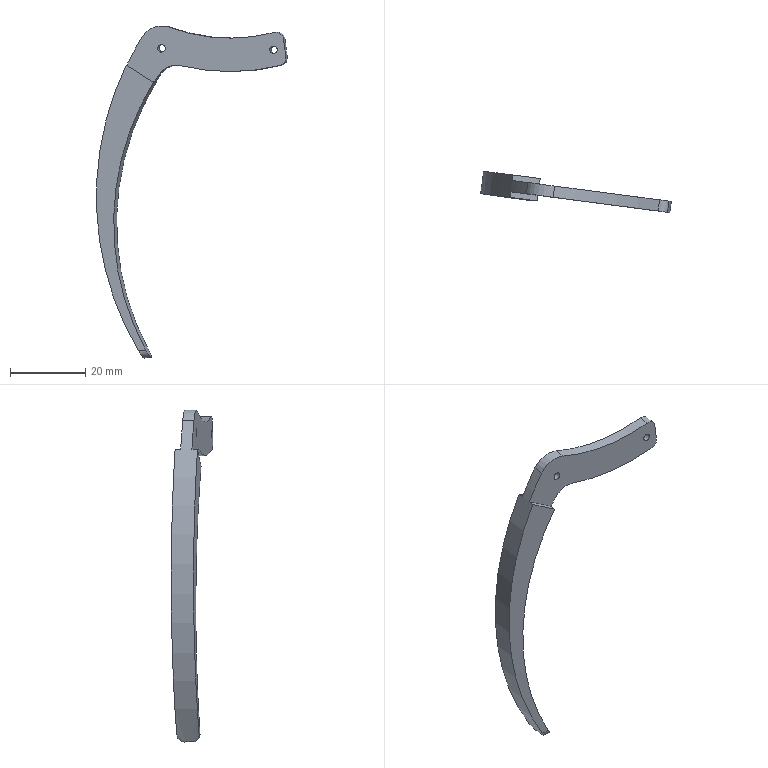Part | NX | features DATUM_CSYS 4, EXTRUDE 3, SKETCH 3, CPROJ 2, BLEND 1 | 1 solid | 20 faces | box 50.786 x 11.051 x 88.315 mm | volume 3379 mm3 | cylinder 12 | plane 8 | commonest cylinder face diameters 4 x4 2 x2 10.7 x1 12 x1 94.72 x1 112.5 x1
STEP:
#1=CARTESIAN_POINT('',(-233.818,36.549,339.632));
#2=VERTEX_POINT('',#1);
#3=CARTESIAN_POINT('',(-237.962,37.093,332.031));
#4=VERTEX_POINT('',#3);
#5=CARTESIAN_POINT('',(-166.053,27.654,297.099));
#6=DIRECTION('',(0.1302,0.9915,-0.000002994));
#7=DIRECTION('',(-0.9915,0.1302,0.));
#8=AXIS2_PLACEMENT_3D('',#5,#6,#7);
#9=CIRCLE('',#8,80.5);
#10=EDGE_CURVE('',#2,#4,#9,.F.);
#11=ORIENTED_EDGE('',*,*,#10,.T.);
#12=CARTESIAN_POINT('',(-237.767,38.58,332.031));
#13=VERTEX_POINT('',#12);
#14=CARTESIAN_POINT('',(-238.547,32.631,332.031));
#15=DIRECTION('',(0.1302,0.9915,-0.000002994));
#16=VECTOR('',#15,1000.);
#17=LINE('',#14,#16);
#18=EDGE_CURVE('',#4,#13,#17,.T.);
#19=ORIENTED_EDGE('',*,*,#18,.T.);
#20=CARTESIAN_POINT('',(-234.495,38.151,256.014));
#21=VERTEX_POINT('',#20);
#22=CARTESIAN_POINT('',(-165.858,29.141,297.099));
#23=DIRECTION('',(0.1302,0.9915,-0.000002994));
#24=DIRECTION('',(0.9915,-0.1302,0.));
#25=AXIS2_PLACEMENT_3D('',#22,#23,#24);
#26=CIRCLE('',#25,80.5);
#27=EDGE_CURVE('',#21,#13,#26,.T.);
#28=ORIENTED_EDGE('',*,*,#27,.F.);
#29=CARTESIAN_POINT('',(-233.623,36.019,254.147));
#30=VERTEX_POINT('',#29);
#31=CARTESIAN_POINT('',(-234.495,38.151,256.014));
#32=CARTESIAN_POINT('',(-234.215,38.114,255.539));
#33=CARTESIAN_POINT('',(-233.699,37.656,254.602));
#34=CARTESIAN_POINT('',(-233.55,36.569,254.147));
#35=CARTESIAN_POINT('',(-233.623,36.019,254.147));
#36=B_SPLINE_CURVE_WITH_KNOTS('',3,(#31,#32,#33,#34,#35),.UNSPECIFIED.,.F.,.F.,(4,1,4),(0.,0.001636,0.003273),.UNSPECIFIED.);
#37=EDGE_CURVE('',#21,#30,#36,.T.);
#38=ORIENTED_EDGE('',*,*,#37,.T.);
#39=CARTESIAN_POINT('',(-233.883,34.036,254.147));
#40=VERTEX_POINT('',#39);
#41=CARTESIAN_POINT('',(-234.143,32.053,254.147));
#42=DIRECTION('',(0.1302,0.9915,-0.000002994));
#43=VECTOR('',#42,1000.);
#44=LINE('',#41,#43);
#45=EDGE_CURVE('',#40,#30,#44,.T.);
#46=ORIENTED_EDGE('',*,*,#45,.F.);
#47=CARTESIAN_POINT('',(-235.276,32.202,256.014));
#48=VERTEX_POINT('',#47);
#49=CARTESIAN_POINT('',(-233.883,34.036,254.147));
#50=CARTESIAN_POINT('',(-233.955,33.487,254.147));
#51=CARTESIAN_POINT('',(-234.378,32.476,254.6));
#52=CARTESIAN_POINT('',(-234.997,32.165,255.539));
#53=CARTESIAN_POINT('',(-235.276,32.202,256.014));
#54=B_SPLINE_CURVE_WITH_KNOTS('',3,(#49,#50,#51,#52,#53),.UNSPECIFIED.,.F.,.F.,(4,1,4),(0.,0.001636,0.003273),.UNSPECIFIED.);
#55=EDGE_CURVE('',#40,#48,#54,.T.);
#56=ORIENTED_EDGE('',*,*,#55,.T.);
#57=CARTESIAN_POINT('',(-238.547,32.631,332.031));
#58=VERTEX_POINT('',#57);
#59=CARTESIAN_POINT('',(-166.639,23.192,297.099));
#60=DIRECTION('',(0.1302,0.9915,-0.000002994));
#61=DIRECTION('',(0.9915,-0.1302,0.));
#62=AXIS2_PLACEMENT_3D('',#59,#60,#61);
#63=CIRCLE('',#62,80.5);
#64=EDGE_CURVE('',#48,#58,#63,.T.);
#65=ORIENTED_EDGE('',*,*,#64,.T.);
#66=CARTESIAN_POINT('',(-238.352,34.119,332.031));
#67=VERTEX_POINT('',#66);
#68=CARTESIAN_POINT('',(-238.547,32.631,332.031));
#69=DIRECTION('',(0.1302,0.9915,-0.000002994));
#70=VECTOR('',#69,1000.);
#71=LINE('',#68,#70);
#72=EDGE_CURVE('',#67,#58,#71,.F.);
#73=ORIENTED_EDGE('',*,*,#72,.F.);
#74=CARTESIAN_POINT('',(-234.208,33.575,339.632));
#75=VERTEX_POINT('',#74);
#76=CARTESIAN_POINT('',(-166.443,24.679,297.099));
#77=DIRECTION('',(0.1302,0.9915,-0.000002994));
#78=DIRECTION('',(-0.9915,0.1302,0.));
#79=AXIS2_PLACEMENT_3D('',#76,#77,#78);
#80=CIRCLE('',#79,80.5);
#81=EDGE_CURVE('',#75,#67,#80,.F.);
#82=ORIENTED_EDGE('',*,*,#81,.F.);
#83=CARTESIAN_POINT('',(-234.403,32.087,339.632));
#84=DIRECTION('',(0.1302,0.9915,-0.000002994));
#85=VECTOR('',#84,1000.);
#86=LINE('',#83,#85);
#87=EDGE_CURVE('',#75,#2,#86,.T.);
#88=ORIENTED_EDGE('',*,*,#87,.T.);
#89=EDGE_LOOP('',(#11,#19,#28,#38,#46,#56,#65,#73,#82,#88));
#90=FACE_BOUND('',#89,.T.);
#91=CARTESIAN_POINT('',(-166.639,23.192,297.099));
#92=DIRECTION('',(0.1302,0.9915,-0.000002994));
#93=DIRECTION('',(-0.9915,0.1302,0.));
#94=AXIS2_PLACEMENT_3D('',#91,#92,#93);
#95=CYLINDRICAL_SURFACE('',#94,80.5);
#96=ADVANCED_FACE('',(#90),#95,.T.);
#97=CARTESIAN_POINT('',(-227.109,32.643,342.095));
#98=VERTEX_POINT('',#97);
#99=CARTESIAN_POINT('',(-226.718,35.617,342.095));
#100=VERTEX_POINT('',#99);
#101=CARTESIAN_POINT('',(-227.304,31.156,342.095));
#102=DIRECTION('',(0.1302,0.9915,-0.000002994));
#103=VECTOR('',#102,1000.);
#104=LINE('',#101,#103);
#105=EDGE_CURVE('',#98,#100,#104,.T.);
#106=ORIENTED_EDGE('',*,*,#105,.T.);
#107=CARTESIAN_POINT('',(-228.767,35.886,336.462));
#108=DIRECTION('',(0.1302,0.9915,-0.000002994));
#109=DIRECTION('',(-0.9915,0.1302,0.));
#110=AXIS2_PLACEMENT_3D('',#107,#108,#109);
#111=CIRCLE('',#110,6.);
#112=EDGE_CURVE('',#100,#2,#111,.F.);
#113=ORIENTED_EDGE('',*,*,#112,.T.);
#114=ORIENTED_EDGE('',*,*,#87,.F.);
#115=CARTESIAN_POINT('',(-229.157,32.912,336.462));
#116=DIRECTION('',(0.1302,0.9915,-0.000002994));
#117=DIRECTION('',(-0.9915,0.1302,0.));
#118=AXIS2_PLACEMENT_3D('',#115,#116,#117);
#119=CIRCLE('',#118,6.);
#120=EDGE_CURVE('',#98,#75,#119,.F.);
#121=ORIENTED_EDGE('',*,*,#120,.F.);
#122=EDGE_LOOP('',(#106,#113,#114,#121));
#123=FACE_BOUND('',#122,.T.);
#124=CARTESIAN_POINT('',(-229.352,31.424,336.462));
#125=DIRECTION('',(0.1302,0.9915,-0.000002994));
#126=DIRECTION('',(-0.9915,0.1302,0.));
#127=AXIS2_PLACEMENT_3D('',#124,#125,#126);
#128=CYLINDRICAL_SURFACE('',#127,6.);
#129=ADVANCED_FACE('',(#123),#128,.T.);
#130=CARTESIAN_POINT('',(-199.174,28.976,340.71));
#131=VERTEX_POINT('',#130);
#132=CARTESIAN_POINT('',(-198.783,31.95,340.71));
#133=VERTEX_POINT('',#132);
#134=CARTESIAN_POINT('',(-199.369,27.488,340.71));
#135=DIRECTION('',(0.1302,0.9915,-0.000002994));
#136=VECTOR('',#135,1000.);
#137=LINE('',#134,#136);
#138=EDGE_CURVE('',#131,#133,#137,.T.);
#139=ORIENTED_EDGE('',*,*,#138,.T.);
#140=CARTESIAN_POINT('',(-210.55,33.495,386.559));
#141=DIRECTION('',(0.1302,0.9915,-0.000002994));
#142=DIRECTION('',(-0.9915,0.1302,0.));
#143=AXIS2_PLACEMENT_3D('',#140,#141,#142);
#144=CIRCLE('',#143,47.36);
#145=EDGE_CURVE('',#133,#100,#144,.T.);
#146=ORIENTED_EDGE('',*,*,#145,.T.);
#147=ORIENTED_EDGE('',*,*,#105,.F.);
#148=CARTESIAN_POINT('',(-210.94,30.521,386.559));
#149=DIRECTION('',(0.1302,0.9915,-0.000002994));
#150=DIRECTION('',(-0.9915,0.1302,0.));
#151=AXIS2_PLACEMENT_3D('',#148,#149,#150);
#152=CIRCLE('',#151,47.36);
#153=EDGE_CURVE('',#131,#98,#152,.T.);
#154=ORIENTED_EDGE('',*,*,#153,.F.);
#155=EDGE_LOOP('',(#139,#146,#147,#154));
#156=FACE_BOUND('',#155,.T.);
#157=CARTESIAN_POINT('',(-211.135,29.033,386.559));
#158=DIRECTION('',(0.1302,0.9915,-0.000002994));
#159=DIRECTION('',(-0.9915,0.1302,0.));
#160=AXIS2_PLACEMENT_3D('',#157,#158,#159);
#161=CYLINDRICAL_SURFACE('',#160,47.36);
#162=ADVANCED_FACE('',(#156),#161,.F.);
#163=CARTESIAN_POINT('',(-196.71,28.652,339.034));
#164=VERTEX_POINT('',#163);
#165=CARTESIAN_POINT('',(-196.32,31.627,339.034));
#166=VERTEX_POINT('',#165);
#167=CARTESIAN_POINT('',(-196.906,27.165,339.034));
#168=DIRECTION('',(0.1302,0.9915,-0.000002994));
#169=VECTOR('',#168,1000.);
#170=LINE('',#167,#169);
#171=EDGE_CURVE('',#164,#166,#170,.T.);
#172=ORIENTED_EDGE('',*,*,#171,.T.);
#173=CARTESIAN_POINT('',(-198.286,31.885,338.774));
#174=DIRECTION('',(0.1302,0.9915,-0.000002994));
#175=DIRECTION('',(-0.9915,0.1302,0.));
#176=AXIS2_PLACEMENT_3D('',#173,#174,#175);
#177=CIRCLE('',#176,2.);
#178=EDGE_CURVE('',#166,#133,#177,.F.);
#179=ORIENTED_EDGE('',*,*,#178,.T.);
#180=ORIENTED_EDGE('',*,*,#138,.F.);
#181=CARTESIAN_POINT('',(-198.677,28.911,338.774));
#182=DIRECTION('',(0.1302,0.9915,-0.000002994));
#183=DIRECTION('',(-0.9915,0.1302,0.));
#184=AXIS2_PLACEMENT_3D('',#181,#182,#183);
#185=CIRCLE('',#184,2.);
#186=EDGE_CURVE('',#164,#131,#185,.F.);
#187=ORIENTED_EDGE('',*,*,#186,.F.);
#188=EDGE_LOOP('',(#172,#179,#180,#187));
#189=FACE_BOUND('',#188,.T.);
#190=CARTESIAN_POINT('',(-198.872,27.423,338.774));
#191=DIRECTION('',(0.1302,0.9915,-0.000002994));
#192=DIRECTION('',(-0.9915,0.1302,0.));
#193=AXIS2_PLACEMENT_3D('',#190,#191,#192);
#194=CYLINDRICAL_SURFACE('',#193,2.);
#195=ADVANCED_FACE('',(#189),#194,.T.);
#196=CARTESIAN_POINT('',(-196.075,28.569,334.153));
#197=VERTEX_POINT('',#196);
#198=CARTESIAN_POINT('',(-195.685,31.543,334.153));
#199=VERTEX_POINT('',#198);
#200=CARTESIAN_POINT('',(-196.27,27.082,334.153));
#201=DIRECTION('',(0.1302,0.9915,-0.000002994));
#202=VECTOR('',#201,1000.);
#203=LINE('',#200,#202);
#204=EDGE_CURVE('',#197,#199,#203,.T.);
#205=ORIENTED_EDGE('',*,*,#204,.T.);
#206=CARTESIAN_POINT('',(-196.32,31.627,339.034));
#207=DIRECTION('',(-0.129,0.01694,0.9915));
#208=VECTOR('',#207,1000.);
#209=LINE('',#206,#208);
#210=EDGE_CURVE('',#199,#166,#209,.T.);
#211=ORIENTED_EDGE('',*,*,#210,.T.);
#212=ORIENTED_EDGE('',*,*,#171,.F.);
#213=CARTESIAN_POINT('',(-196.71,28.652,339.034));
#214=DIRECTION('',(-0.129,0.01694,0.9915));
#215=VECTOR('',#214,1000.);
#216=LINE('',#213,#215);
#217=EDGE_CURVE('',#197,#164,#216,.T.);
#218=ORIENTED_EDGE('',*,*,#217,.F.);
#219=EDGE_LOOP('',(#205,#211,#212,#218));
#220=FACE_BOUND('',#219,.T.);
#221=CARTESIAN_POINT('',(-196.906,27.165,339.034));
#222=DIRECTION('',(0.9831,-0.129,0.1302));
#223=DIRECTION('',(0.1313,0.,-0.9913));
#224=AXIS2_PLACEMENT_3D('',#221,#222,#223);
#225=PLANE('',#224);
#226=ADVANCED_FACE('',(#220),#225,.T.);
#227=CARTESIAN_POINT('',(-197.566,28.765,331.951));
#228=VERTEX_POINT('',#227);
#229=CARTESIAN_POINT('',(-197.175,31.739,331.951));
#230=VERTEX_POINT('',#229);
#231=CARTESIAN_POINT('',(-197.761,27.277,331.951));
#232=DIRECTION('',(0.1302,0.9915,-0.000002994));
#233=VECTOR('',#232,1000.);
#234=LINE('',#231,#233);
#235=EDGE_CURVE('',#228,#230,#234,.T.);
#236=ORIENTED_EDGE('',*,*,#235,.T.);
#237=CARTESIAN_POINT('',(-197.651,31.802,333.892));
#238=DIRECTION('',(0.1302,0.9915,-0.000002994));
#239=DIRECTION('',(-0.9915,0.1302,0.));
#240=AXIS2_PLACEMENT_3D('',#237,#238,#239);
#241=CIRCLE('',#240,2.);
#242=EDGE_CURVE('',#230,#199,#241,.F.);
#243=ORIENTED_EDGE('',*,*,#242,.T.);
#244=ORIENTED_EDGE('',*,*,#204,.F.);
#245=CARTESIAN_POINT('',(-198.041,28.827,333.892));
#246=DIRECTION('',(0.1302,0.9915,-0.000002994));
#247=DIRECTION('',(-0.9915,0.1302,0.));
#248=AXIS2_PLACEMENT_3D('',#245,#246,#247);
#249=CIRCLE('',#248,2.);
#250=EDGE_CURVE('',#228,#197,#249,.F.);
#251=ORIENTED_EDGE('',*,*,#250,.F.);
#252=EDGE_LOOP('',(#236,#243,#244,#251));
#253=FACE_BOUND('',#252,.T.);
#254=CARTESIAN_POINT('',(-198.236,27.34,333.892));
#255=DIRECTION('',(0.1302,0.9915,-0.000002994));
#256=DIRECTION('',(-0.9915,0.1302,0.));
#257=AXIS2_PLACEMENT_3D('',#254,#255,#256);
#258=CYLINDRICAL_SURFACE('',#257,2.);
#259=ADVANCED_FACE('',(#253),#258,.T.);
#260=CARTESIAN_POINT('',(-224.029,32.239,331.88));
#261=VERTEX_POINT('',#260);
#262=CARTESIAN_POINT('',(-223.639,35.213,331.88));
#263=VERTEX_POINT('',#262);
#264=CARTESIAN_POINT('',(-224.225,30.751,331.88));
#265=DIRECTION('',(0.1302,0.9915,-0.000002994));
#266=VECTOR('',#265,1000.);
#267=LINE('',#264,#266);
#268=EDGE_CURVE('',#261,#263,#267,.T.);
#269=ORIENTED_EDGE('',*,*,#268,.T.);
#270=CARTESIAN_POINT('',(-210.55,33.495,386.559));
#271=DIRECTION('',(0.1302,0.9915,-0.000002994));
#272=DIRECTION('',(-0.9915,0.1302,0.));
#273=AXIS2_PLACEMENT_3D('',#270,#271,#272);
#274=CIRCLE('',#273,56.25);
#275=EDGE_CURVE('',#263,#230,#274,.F.);
#276=ORIENTED_EDGE('',*,*,#275,.T.);
#277=ORIENTED_EDGE('',*,*,#235,.F.);
#278=CARTESIAN_POINT('',(-210.94,30.521,386.559));
#279=DIRECTION('',(0.1302,0.9915,-0.000002994));
#280=DIRECTION('',(-0.9915,0.1302,0.));
#281=AXIS2_PLACEMENT_3D('',#278,#279,#280);
#282=CIRCLE('',#281,56.25);
#283=EDGE_CURVE('',#261,#228,#282,.F.);
#284=ORIENTED_EDGE('',*,*,#283,.F.);
#285=EDGE_LOOP('',(#269,#276,#277,#284));
#286=FACE_BOUND('',#285,.T.);
#287=CARTESIAN_POINT('',(-211.135,29.033,386.559));
#288=DIRECTION('',(0.1302,0.9915,-0.000002994));
#289=DIRECTION('',(-0.9915,0.1302,0.));
#290=AXIS2_PLACEMENT_3D('',#287,#288,#289);
#291=CYLINDRICAL_SURFACE('',#290,56.25);
#292=ADVANCED_FACE('',(#286),#291,.T.);
#293=CARTESIAN_POINT('',(-229.676,32.98,329.666));
#294=VERTEX_POINT('',#293);
#295=CARTESIAN_POINT('',(-229.285,35.954,329.666));
#296=VERTEX_POINT('',#295);
#297=CARTESIAN_POINT('',(-229.871,31.493,329.666));
#298=DIRECTION('',(0.1302,0.9915,-0.000002994));
#299=VECTOR('',#298,1000.);
#300=LINE('',#297,#299);
#301=EDGE_CURVE('',#294,#296,#300,.T.);
#302=ORIENTED_EDGE('',*,*,#301,.T.);
#303=CARTESIAN_POINT('',(-224.884,35.376,326.68));
#304=DIRECTION('',(0.1302,0.9915,-0.000002994));
#305=DIRECTION('',(-0.9915,0.1302,0.));
#306=AXIS2_PLACEMENT_3D('',#303,#304,#305);
#307=CIRCLE('',#306,5.35);
#308=EDGE_CURVE('',#296,#263,#307,.T.);
#309=ORIENTED_EDGE('',*,*,#308,.T.);
#310=ORIENTED_EDGE('',*,*,#268,.F.);
#311=CARTESIAN_POINT('',(-225.274,32.402,326.68));
#312=DIRECTION('',(0.1302,0.9915,-0.000002994));
#313=DIRECTION('',(-0.9915,0.1302,0.));
#314=AXIS2_PLACEMENT_3D('',#311,#312,#313);
#315=CIRCLE('',#314,5.35);
#316=EDGE_CURVE('',#294,#261,#315,.T.);
#317=ORIENTED_EDGE('',*,*,#316,.F.);
#318=EDGE_LOOP('',(#302,#309,#310,#317));
#319=FACE_BOUND('',#318,.T.);
#320=CARTESIAN_POINT('',(-225.469,30.915,326.68));
#321=DIRECTION('',(0.1302,0.9915,-0.000002994));
#322=DIRECTION('',(-0.9915,0.1302,0.));
#323=AXIS2_PLACEMENT_3D('',#320,#321,#322);
#324=CYLINDRICAL_SURFACE('',#323,5.35);
#325=ADVANCED_FACE('',(#319),#324,.F.);
#326=CARTESIAN_POINT('',(-230.547,37.633,327.389));
#327=VERTEX_POINT('',#326);
#328=CARTESIAN_POINT('',(-232.6,37.902,256.265));
#329=VERTEX_POINT('',#328);
#330=CARTESIAN_POINT('',(-170.679,29.774,290.038));
#331=DIRECTION('',(-0.1302,-0.9915,0.000002994));
#332=DIRECTION('',(0.9915,-0.1302,0.));
#333=AXIS2_PLACEMENT_3D('',#330,#331,#332);
#334=CIRCLE('',#333,71.);
#335=EDGE_CURVE('',#327,#329,#334,.T.);
#336=ORIENTED_EDGE('',*,*,#335,.F.);
#337=CARTESIAN_POINT('',(-230.742,36.145,327.389));
#338=VERTEX_POINT('',#337);
#339=CARTESIAN_POINT('',(-230.156,40.607,327.389));
#340=DIRECTION('',(-0.1302,-0.9915,0.000002994));
#341=VECTOR('',#340,1000.);
#342=LINE('',#339,#341);
#343=EDGE_CURVE('',#327,#338,#342,.T.);
#344=ORIENTED_EDGE('',*,*,#343,.T.);
#345=CARTESIAN_POINT('',(-170.874,28.286,290.038));
#346=DIRECTION('',(0.1302,0.9915,-0.000002994));
#347=DIRECTION('',(-0.9915,0.1302,0.));
#348=AXIS2_PLACEMENT_3D('',#345,#346,#347);
#349=CIRCLE('',#348,71.);
#350=EDGE_CURVE('',#338,#296,#349,.T.);
#351=ORIENTED_EDGE('',*,*,#350,.T.);
#352=ORIENTED_EDGE('',*,*,#301,.F.);
#353=CARTESIAN_POINT('',(-231.132,33.171,327.389));
#354=VERTEX_POINT('',#353);
#355=CARTESIAN_POINT('',(-171.264,25.312,290.038));
#356=DIRECTION('',(0.1302,0.9915,-0.000002994));
#357=DIRECTION('',(-0.9915,0.1302,0.));
#358=AXIS2_PLACEMENT_3D('',#355,#356,#357);
#359=CIRCLE('',#358,71.);
#360=EDGE_CURVE('',#354,#294,#359,.T.);
#361=ORIENTED_EDGE('',*,*,#360,.F.);
#362=CARTESIAN_POINT('',(-231.328,31.684,327.389));
#363=VERTEX_POINT('',#362);
#364=CARTESIAN_POINT('',(-231.718,28.709,327.389));
#365=DIRECTION('',(0.1302,0.9915,-0.000002994));
#366=VECTOR('',#365,1000.);
#367=LINE('',#364,#366);
#368=EDGE_CURVE('',#363,#354,#367,.T.);
#369=ORIENTED_EDGE('',*,*,#368,.F.);
#370=CARTESIAN_POINT('',(-233.381,31.953,256.265));
#371=VERTEX_POINT('',#370);
#372=CARTESIAN_POINT('',(-171.46,23.825,290.038));
#373=DIRECTION('',(-0.1302,-0.9915,0.000002994));
#374=DIRECTION('',(0.9915,-0.1302,0.));
#375=AXIS2_PLACEMENT_3D('',#372,#373,#374);
#376=CIRCLE('',#375,71.);
#377=EDGE_CURVE('',#363,#371,#376,.T.);
#378=ORIENTED_EDGE('',*,*,#377,.T.);
#379=CARTESIAN_POINT('',(-232.077,33.799,254.386));
#380=VERTEX_POINT('',#379);
#381=CARTESIAN_POINT('',(-233.381,31.953,256.265));
#382=CARTESIAN_POINT('',(-233.123,31.919,255.783));
#383=CARTESIAN_POINT('',(-232.546,32.243,254.835));
#384=CARTESIAN_POINT('',(-232.148,33.254,254.386));
#385=CARTESIAN_POINT('',(-232.077,33.799,254.386));
#386=B_SPLINE_CURVE_WITH_KNOTS('',3,(#381,#382,#383,#384,#385),.UNSPECIFIED.,.F.,.F.,(4,1,4),(0.,0.001622,0.003245),.UNSPECIFIED.);
#387=EDGE_CURVE('',#371,#380,#386,.T.);
#388=ORIENTED_EDGE('',*,*,#387,.T.);
#389=CARTESIAN_POINT('',(-231.816,35.782,254.386));
#390=VERTEX_POINT('',#389);
#391=CARTESIAN_POINT('',(-232.337,31.816,254.386));
#392=DIRECTION('',(0.1302,0.9915,-0.000002994));
#393=VECTOR('',#392,1000.);
#394=LINE('',#391,#393);
#395=EDGE_CURVE('',#380,#390,#394,.T.);
#396=ORIENTED_EDGE('',*,*,#395,.T.);
#397=CARTESIAN_POINT('',(-231.816,35.782,254.386));
#398=CARTESIAN_POINT('',(-231.745,36.326,254.386));
#399=CARTESIAN_POINT('',(-231.867,37.405,254.833));
#400=CARTESIAN_POINT('',(-232.342,37.868,255.783));
#401=CARTESIAN_POINT('',(-232.6,37.902,256.265));
#402=B_SPLINE_CURVE_WITH_KNOTS('',3,(#397,#398,#399,#400,#401),.UNSPECIFIED.,.F.,.F.,(4,1,4),(0.,0.001622,0.003245),.UNSPECIFIED.);
#403=EDGE_CURVE('',#390,#329,#402,.T.);
#404=ORIENTED_EDGE('',*,*,#403,.T.);
#405=EDGE_LOOP('',(#336,#344,#351,#352,#361,#369,#378,#388,#396,#404));
#406=FACE_BOUND('',#405,.T.);
#407=CARTESIAN_POINT('',(-171.46,23.825,290.038));
#408=DIRECTION('',(0.1302,0.9915,-0.000002994));
#409=DIRECTION('',(-0.9915,0.1302,0.));
#410=AXIS2_PLACEMENT_3D('',#407,#408,#409);
#411=CYLINDRICAL_SURFACE('',#410,71.);
#412=ADVANCED_FACE('',(#406),#411,.F.);
#413=CARTESIAN_POINT('',(-230.149,33.042,336.462));
#414=VERTEX_POINT('',#413);
#415=CARTESIAN_POINT('',(-229.157,32.912,336.462));
#416=DIRECTION('',(0.1302,0.9915,-0.000002994));
#417=DIRECTION('',(-0.9915,0.1302,0.));
#418=AXIS2_PLACEMENT_3D('',#415,#416,#417);
#419=CIRCLE('',#418,1.);
#420=EDGE_CURVE('',#414,#414,#419,.F.);
#421=ORIENTED_EDGE('',*,*,#420,.T.);
#422=EDGE_LOOP('',(#421));
#423=FACE_BOUND('',#422,.T.);
#424=CARTESIAN_POINT('',(-229.758,36.016,336.462));
#425=VERTEX_POINT('',#424);
#426=CARTESIAN_POINT('',(-228.767,35.886,336.462));
#427=DIRECTION('',(0.1302,0.9915,-0.000002994));
#428=DIRECTION('',(-0.9915,0.1302,0.));
#429=AXIS2_PLACEMENT_3D('',#426,#427,#428);
#430=CIRCLE('',#429,1.);
#431=EDGE_CURVE('',#425,#425,#430,.F.);
#432=ORIENTED_EDGE('',*,*,#431,.F.);
#433=EDGE_LOOP('',(#432));
#434=FACE_BOUND('',#433,.T.);
#435=CARTESIAN_POINT('',(-229.352,31.424,336.462));
#436=DIRECTION('',(0.1302,0.9915,-0.000002994));
#437=DIRECTION('',(-0.9915,0.1302,0.));
#438=AXIS2_PLACEMENT_3D('',#435,#436,#437);
#439=CYLINDRICAL_SURFACE('',#438,1.);
#440=ADVANCED_FACE('',(#423,#434),#439,.F.);
#441=CARTESIAN_POINT('',(-200.32,29.126,336.1));
#442=VERTEX_POINT('',#441);
#443=CARTESIAN_POINT('',(-199.329,28.996,336.1));
#444=DIRECTION('',(0.1302,0.9915,-0.000002994));
#445=DIRECTION('',(-0.9915,0.1302,0.));
#446=AXIS2_PLACEMENT_3D('',#443,#444,#445);
#447=CIRCLE('',#446,1.);
#448=EDGE_CURVE('',#442,#442,#447,.F.);
#449=ORIENTED_EDGE('',*,*,#448,.T.);
#450=EDGE_LOOP('',(#449));
#451=FACE_BOUND('',#450,.T.);
#452=CARTESIAN_POINT('',(-199.93,32.101,336.1));
#453=VERTEX_POINT('',#452);
#454=CARTESIAN_POINT('',(-198.938,31.971,336.1));
#455=DIRECTION('',(0.1302,0.9915,-0.000002994));
#456=DIRECTION('',(-0.9915,0.1302,0.));
#457=AXIS2_PLACEMENT_3D('',#454,#455,#456);
#458=CIRCLE('',#457,1.);
#459=EDGE_CURVE('',#453,#453,#458,.F.);
#460=ORIENTED_EDGE('',*,*,#459,.F.);
#461=EDGE_LOOP('',(#460));
#462=FACE_BOUND('',#461,.T.);
#463=CARTESIAN_POINT('',(-199.524,27.509,336.1));
#464=DIRECTION('',(0.1302,0.9915,-0.000002994));
#465=DIRECTION('',(-0.9915,0.1302,0.));
#466=AXIS2_PLACEMENT_3D('',#463,#464,#465);
#467=CYLINDRICAL_SURFACE('',#466,1.);
#468=ADVANCED_FACE('',(#451,#462),#467,.F.);
#469=ORIENTED_EDGE('',*,*,#27,.T.);
#470=CARTESIAN_POINT('',(-170.941,29.808,289.058));
#471=DIRECTION('',(0.836,-0.1097,-0.5376));
#472=VECTOR('',#471,1000.);
#473=LINE('',#470,#472);
#474=EDGE_CURVE('',#13,#327,#473,.T.);
#475=ORIENTED_EDGE('',*,*,#474,.T.);
#476=ORIENTED_EDGE('',*,*,#335,.T.);
#477=CARTESIAN_POINT('',(-161.764,28.603,265.644));
#478=DIRECTION('',(-0.9831,0.129,-0.1302));
#479=VECTOR('',#478,1000.);
#480=LINE('',#477,#479);
#481=EDGE_CURVE('',#329,#21,#480,.T.);
#482=ORIENTED_EDGE('',*,*,#481,.T.);
#483=EDGE_LOOP('',(#469,#475,#476,#482));
#484=FACE_BOUND('',#483,.T.);
#485=CARTESIAN_POINT('',(-165.858,29.141,297.099));
#486=DIRECTION('',(0.1302,0.9915,-0.000002994));
#487=DIRECTION('',(-0.9915,0.1302,0.));
#488=AXIS2_PLACEMENT_3D('',#485,#486,#487);
#489=PLANE('',#488);
#490=ADVANCED_FACE('',(#484),#489,.T.);
#491=ORIENTED_EDGE('',*,*,#45,.T.);
#492=CARTESIAN_POINT('',(-231.816,35.782,254.386));
#493=DIRECTION('',(-0.9831,0.129,-0.1302));
#494=VECTOR('',#493,1000.);
#495=LINE('',#492,#494);
#496=EDGE_CURVE('',#30,#390,#495,.F.);
#497=ORIENTED_EDGE('',*,*,#496,.T.);
#498=ORIENTED_EDGE('',*,*,#395,.F.);
#499=CARTESIAN_POINT('',(-233.883,34.036,254.147));
#500=DIRECTION('',(-0.9831,0.129,-0.1302));
#501=VECTOR('',#500,1000.);
#502=LINE('',#499,#501);
#503=EDGE_CURVE('',#380,#40,#502,.T.);
#504=ORIENTED_EDGE('',*,*,#503,.T.);
#505=EDGE_LOOP('',(#491,#497,#498,#504));
#506=FACE_BOUND('',#505,.T.);
#507=CARTESIAN_POINT('',(-232.337,31.816,254.386));
#508=DIRECTION('',(0.129,-0.01694,-0.9915));
#509=DIRECTION('',(-0.9916,0.,-0.1291));
#510=AXIS2_PLACEMENT_3D('',#507,#508,#509);
#511=PLANE('',#510);
#512=ADVANCED_FACE('',(#506),#511,.T.);
#513=ORIENTED_EDGE('',*,*,#377,.F.);
#514=CARTESIAN_POINT('',(-171.722,23.859,289.058));
#515=DIRECTION('',(-0.836,0.1097,0.5376));
#516=VECTOR('',#515,1000.);
#517=LINE('',#514,#516);
#518=EDGE_CURVE('',#363,#58,#517,.T.);
#519=ORIENTED_EDGE('',*,*,#518,.T.);
#520=ORIENTED_EDGE('',*,*,#64,.F.);
#521=CARTESIAN_POINT('',(-232.595,31.85,256.369));
#522=DIRECTION('',(-0.9831,0.129,-0.1302));
#523=VECTOR('',#522,1000.);
#524=LINE('',#521,#523);
#525=EDGE_CURVE('',#48,#371,#524,.F.);
#526=ORIENTED_EDGE('',*,*,#525,.T.);
#527=EDGE_LOOP('',(#513,#519,#520,#526));
#528=FACE_BOUND('',#527,.T.);
#529=CARTESIAN_POINT('',(-166.639,23.192,297.099));
#530=DIRECTION('',(0.1302,0.9915,-0.000002994));
#531=DIRECTION('',(-0.9915,0.1302,0.));
#532=AXIS2_PLACEMENT_3D('',#529,#530,#531);
#533=PLANE('',#532);
#534=ADVANCED_FACE('',(#528),#533,.F.);
#535=ORIENTED_EDGE('',*,*,#403,.F.);
#536=ORIENTED_EDGE('',*,*,#496,.F.);
#537=ORIENTED_EDGE('',*,*,#37,.F.);
#538=ORIENTED_EDGE('',*,*,#481,.F.);
#539=EDGE_LOOP('',(#535,#536,#537,#538));
#540=FACE_BOUND('',#539,.T.);
#541=CARTESIAN_POINT('',(-162.024,26.62,265.644));
#542=DIRECTION('',(-0.9831,0.129,-0.1302));
#543=DIRECTION('',(-0.1313,0.,0.9913));
#544=AXIS2_PLACEMENT_3D('',#541,#542,#543);
#545=CYLINDRICAL_SURFACE('',#544,2.);
#546=ADVANCED_FACE('',(#540),#545,.T.);
#547=ORIENTED_EDGE('',*,*,#387,.F.);
#548=ORIENTED_EDGE('',*,*,#525,.F.);
#549=ORIENTED_EDGE('',*,*,#55,.F.);
#550=ORIENTED_EDGE('',*,*,#503,.F.);
#551=EDGE_LOOP('',(#547,#548,#549,#550));
#552=FACE_BOUND('',#551,.T.);
#553=CARTESIAN_POINT('',(-232.335,33.833,256.369));
#554=DIRECTION('',(0.9831,-0.129,0.1302));
#555=DIRECTION('',(0.1313,0.,-0.9913));
#556=AXIS2_PLACEMENT_3D('',#553,#554,#555);
#557=CYLINDRICAL_SURFACE('',#556,2.);
#558=ADVANCED_FACE('',(#552),#557,.T.);
#559=ORIENTED_EDGE('',*,*,#81,.T.);
#560=CARTESIAN_POINT('',(-231.132,33.171,327.389));
#561=DIRECTION('',(-0.836,0.1097,0.5376));
#562=VECTOR('',#561,1000.);
#563=LINE('',#560,#562);
#564=EDGE_CURVE('',#67,#354,#563,.F.);
#565=ORIENTED_EDGE('',*,*,#564,.T.);
#566=ORIENTED_EDGE('',*,*,#360,.T.);
#567=ORIENTED_EDGE('',*,*,#316,.T.);
#568=ORIENTED_EDGE('',*,*,#283,.T.);
#569=ORIENTED_EDGE('',*,*,#250,.T.);
#570=ORIENTED_EDGE('',*,*,#217,.T.);
#571=ORIENTED_EDGE('',*,*,#186,.T.);
#572=ORIENTED_EDGE('',*,*,#153,.T.);
#573=ORIENTED_EDGE('',*,*,#120,.T.);
#574=EDGE_LOOP('',(#559,#565,#566,#567,#568,#569,#570,#571,#572,#573));
#575=FACE_BOUND('',#574,.T.);
#576=ORIENTED_EDGE('',*,*,#448,.F.);
#577=EDGE_LOOP('',(#576));
#578=FACE_BOUND('',#577,.T.);
#579=ORIENTED_EDGE('',*,*,#420,.F.);
#580=EDGE_LOOP('',(#579));
#581=FACE_BOUND('',#580,.T.);
#582=CARTESIAN_POINT('',(0.3651,2.781,-0.000008398));
#583=DIRECTION('',(0.1302,0.9915,-0.000002994));
#584=DIRECTION('',(-0.9915,0.1302,0.));
#585=AXIS2_PLACEMENT_3D('',#582,#583,#584);
#586=PLANE('',#585);
#587=ADVANCED_FACE('',(#575,#578,#581),#586,.F.);
#588=ORIENTED_EDGE('',*,*,#72,.T.);
#589=ORIENTED_EDGE('',*,*,#518,.F.);
#590=ORIENTED_EDGE('',*,*,#368,.T.);
#591=ORIENTED_EDGE('',*,*,#564,.F.);
#592=EDGE_LOOP('',(#588,#589,#590,#591));
#593=FACE_BOUND('',#592,.T.);
#594=CARTESIAN_POINT('',(-231.718,28.709,327.389));
#595=DIRECTION('',(-0.533,0.06997,-0.8432));
#596=DIRECTION('',(-0.8453,0.,0.5344));
#597=AXIS2_PLACEMENT_3D('',#594,#595,#596);
#598=PLANE('',#597);
#599=ADVANCED_FACE('',(#593),#598,.F.);
#600=ORIENTED_EDGE('',*,*,#112,.F.);
#601=ORIENTED_EDGE('',*,*,#145,.F.);
#602=ORIENTED_EDGE('',*,*,#178,.F.);
#603=ORIENTED_EDGE('',*,*,#210,.F.);
#604=ORIENTED_EDGE('',*,*,#242,.F.);
#605=ORIENTED_EDGE('',*,*,#275,.F.);
#606=ORIENTED_EDGE('',*,*,#308,.F.);
#607=ORIENTED_EDGE('',*,*,#350,.F.);
#608=CARTESIAN_POINT('',(-230.742,36.145,327.389));
#609=DIRECTION('',(-0.836,0.1097,0.5376));
#610=VECTOR('',#609,1000.);
#611=LINE('',#608,#610);
#612=EDGE_CURVE('',#4,#338,#611,.F.);
#613=ORIENTED_EDGE('',*,*,#612,.F.);
#614=ORIENTED_EDGE('',*,*,#10,.F.);
#615=EDGE_LOOP('',(#600,#601,#602,#603,#604,#605,#606,#607,#613,#614));
#616=FACE_BOUND('',#615,.T.);
#617=ORIENTED_EDGE('',*,*,#459,.T.);
#618=EDGE_LOOP('',(#617));
#619=FACE_BOUND('',#618,.T.);
#620=ORIENTED_EDGE('',*,*,#431,.T.);
#621=EDGE_LOOP('',(#620));
#622=FACE_BOUND('',#621,.T.);
#623=CARTESIAN_POINT('',(0.7555,5.756,-0.00001738));
#624=DIRECTION('',(0.1302,0.9915,-0.000002994));
#625=DIRECTION('',(-0.9915,0.1302,0.));
#626=AXIS2_PLACEMENT_3D('',#623,#624,#625);
#627=PLANE('',#626);
#628=ADVANCED_FACE('',(#616,#619,#622),#627,.T.);
#629=ORIENTED_EDGE('',*,*,#612,.T.);
#630=ORIENTED_EDGE('',*,*,#343,.F.);
#631=ORIENTED_EDGE('',*,*,#474,.F.);
#632=ORIENTED_EDGE('',*,*,#18,.F.);
#633=EDGE_LOOP('',(#629,#630,#631,#632));
#634=FACE_BOUND('',#633,.T.);
#635=CARTESIAN_POINT('',(-230.156,40.607,327.389));
#636=DIRECTION('',(0.533,-0.06997,0.8432));
#637=DIRECTION('',(0.8453,0.,-0.5344));
#638=AXIS2_PLACEMENT_3D('',#635,#636,#637);
#639=PLANE('',#638);
#640=ADVANCED_FACE('',(#634),#639,.T.);
#641=CLOSED_SHELL('',(#96,#129,#162,#195,#226,#259,#292,#325,#412,#440,#468,#490,#512,#534,#546,#558,#587,#599,#628,#640));
#642=MANIFOLD_SOLID_BREP('',#641);
#643=(LENGTH_UNIT()NAMED_UNIT(*)SI_UNIT(.MILLI.,.METRE.));
#644=UNCERTAINTY_MEASURE_WITH_UNIT(LENGTH_MEASURE(0.0508),#643,'','');
#645=(NAMED_UNIT(*)PLANE_ANGLE_UNIT()SI_UNIT($,.RADIAN.));
#646=(NAMED_UNIT(*)SI_UNIT($,.STERADIAN.)SOLID_ANGLE_UNIT());
#647=(GEOMETRIC_REPRESENTATION_CONTEXT(3)GLOBAL_UNCERTAINTY_ASSIGNED_CONTEXT((#644))GLOBAL_UNIT_ASSIGNED_CONTEXT((#643,#645,#646))REPRESENTATION_CONTEXT('',''));
#648=ADVANCED_BREP_SHAPE_REPRESENTATION('',(#642),#647);